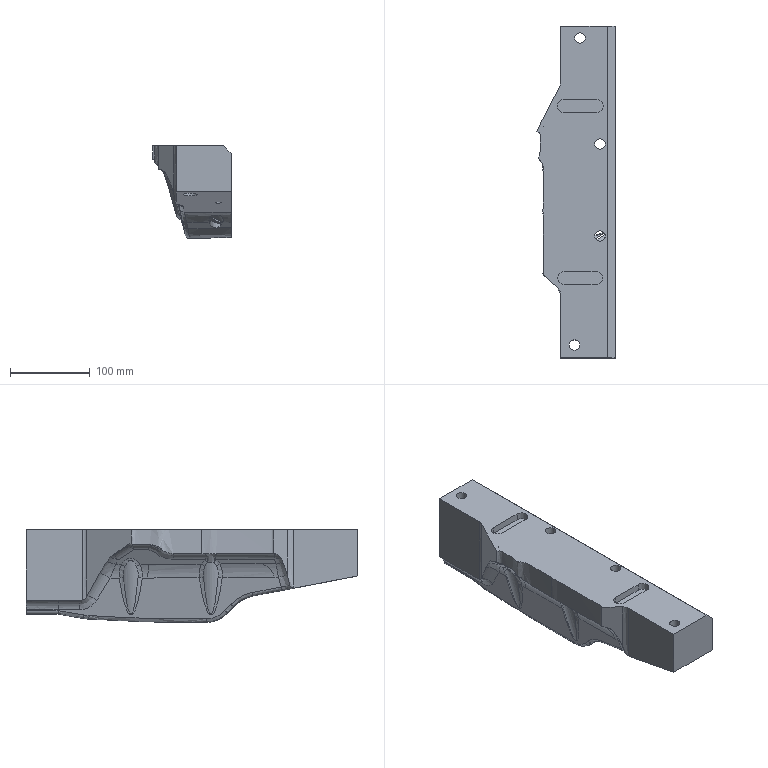Part | NX | features solid 2 | 1 solid | 136 faces | box 98.097 x 415 x 116.547 mm | volume 2735249 mm3 | spline 65 | cylinder 34 | plane 34 | cone 2 | sphere 1 | commonest cylinder face diameters 35 x6 13 x4 16 x4 18.008 x4 29 x4 105 x3